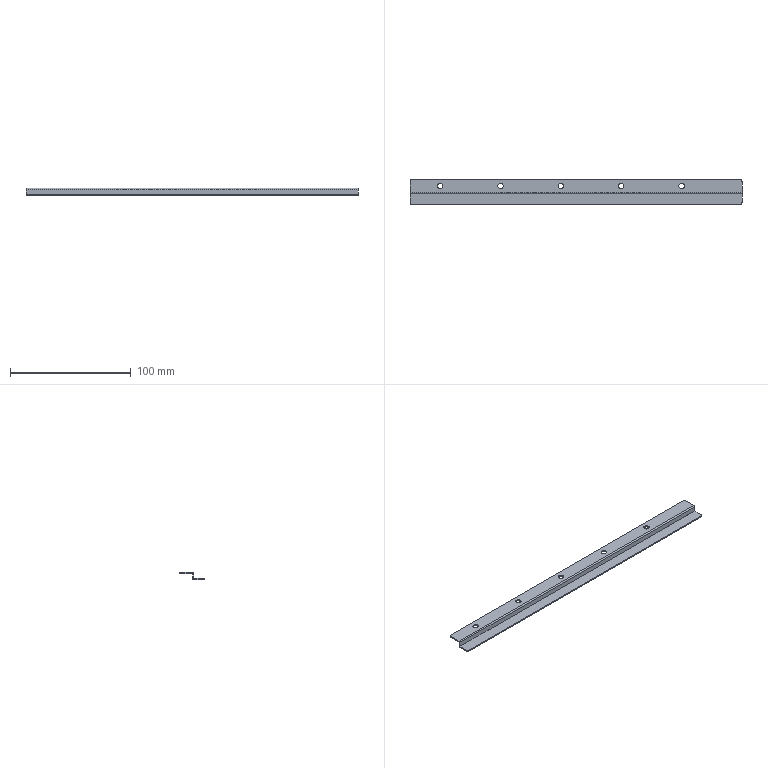Part | STEP file | Cover Reinforcing Rib 275mm | 1 solid | 36 faces | box 275 x 21 x 6 mm | volume 6947 mm3 | cylinder 18 | plane 18 | commonest cylinder face diameters 4.5 x10 4 x4 0.02 x2 2.02 x2